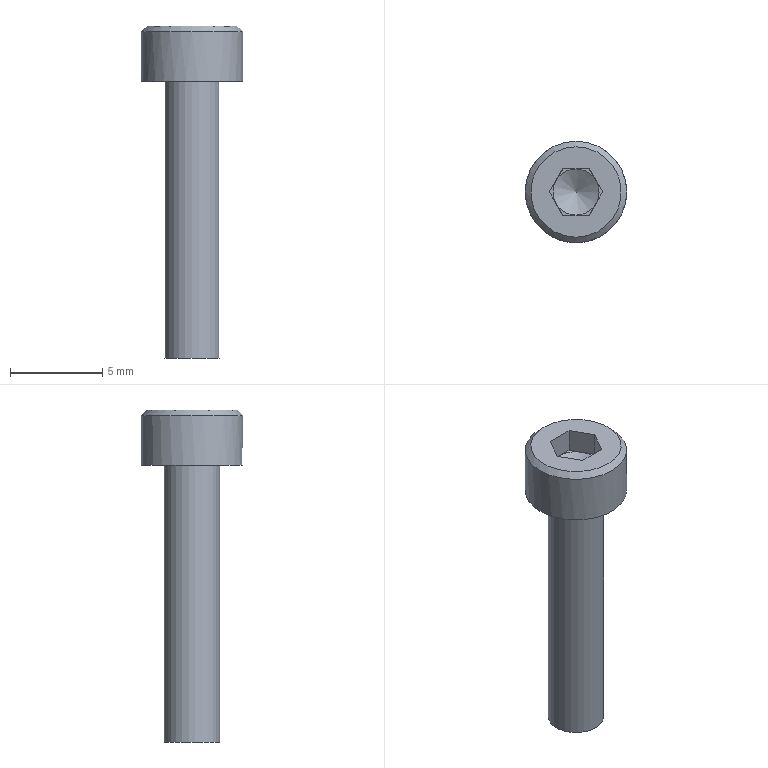Part | NX | features 5003_342_CB3-15 2 | 1 solid | 19 faces | box 5.5 x 5.5 x 18 mm | volume 168.289 mm3 | plane 15 | cylinder 2 | cone 2 | commonest cylinder face diameters 3 x1 5.5 x1
STEP:
#1=CARTESIAN_POINT('',(133.525,-558.45,-190.8));
#2=VERTEX_POINT('',#1);
#3=CARTESIAN_POINT('',(133.525,-556.,-190.8));
#4=DIRECTION('',(0.,0.,-1.));
#5=DIRECTION('',(0.,-1.,0.));
#6=AXIS2_PLACEMENT_3D('',#3,#4,#5);
#7=CIRCLE('',#6,2.45);
#8=EDGE_CURVE('',#2,#2,#7,.F.);
#9=ORIENTED_EDGE('',*,*,#8,.T.);
#10=EDGE_LOOP('',(#9));
#11=FACE_BOUND('',#10,.T.);
#12=CARTESIAN_POINT('',(134.968,-556.,-190.8));
#13=VERTEX_POINT('',#12);
#14=CARTESIAN_POINT('',(134.247,-554.75,-190.8));
#15=VERTEX_POINT('',#14);
#16=CARTESIAN_POINT('',(134.968,-556.,-190.8));
#17=DIRECTION('',(-0.5,0.866,0.));
#18=VECTOR('',#17,1000.);
#19=LINE('',#16,#18);
#20=EDGE_CURVE('',#13,#15,#19,.T.);
#21=ORIENTED_EDGE('',*,*,#20,.F.);
#22=CARTESIAN_POINT('',(134.247,-557.25,-190.8));
#23=VERTEX_POINT('',#22);
#24=CARTESIAN_POINT('',(134.247,-557.25,-190.8));
#25=DIRECTION('',(0.5,0.866,0.));
#26=VECTOR('',#25,1000.);
#27=LINE('',#24,#26);
#28=EDGE_CURVE('',#23,#13,#27,.T.);
#29=ORIENTED_EDGE('',*,*,#28,.F.);
#30=CARTESIAN_POINT('',(132.803,-557.25,-190.8));
#31=VERTEX_POINT('',#30);
#32=CARTESIAN_POINT('',(132.803,-557.25,-190.8));
#33=DIRECTION('',(1.,0.,0.));
#34=VECTOR('',#33,1000.);
#35=LINE('',#32,#34);
#36=EDGE_CURVE('',#31,#23,#35,.T.);
#37=ORIENTED_EDGE('',*,*,#36,.F.);
#38=CARTESIAN_POINT('',(132.082,-556.,-190.8));
#39=VERTEX_POINT('',#38);
#40=CARTESIAN_POINT('',(132.082,-556.,-190.8));
#41=DIRECTION('',(0.5,-0.866,0.));
#42=VECTOR('',#41,1000.);
#43=LINE('',#40,#42);
#44=EDGE_CURVE('',#39,#31,#43,.T.);
#45=ORIENTED_EDGE('',*,*,#44,.F.);
#46=CARTESIAN_POINT('',(132.803,-554.75,-190.8));
#47=VERTEX_POINT('',#46);
#48=CARTESIAN_POINT('',(132.803,-554.75,-190.8));
#49=DIRECTION('',(-0.5,-0.866,0.));
#50=VECTOR('',#49,1000.);
#51=LINE('',#48,#50);
#52=EDGE_CURVE('',#47,#39,#51,.T.);
#53=ORIENTED_EDGE('',*,*,#52,.F.);
#54=CARTESIAN_POINT('',(134.247,-554.75,-190.8));
#55=DIRECTION('',(-1.,0.,0.));
#56=VECTOR('',#55,1000.);
#57=LINE('',#54,#56);
#58=EDGE_CURVE('',#15,#47,#57,.T.);
#59=ORIENTED_EDGE('',*,*,#58,.F.);
#60=EDGE_LOOP('',(#21,#29,#37,#45,#53,#59));
#61=FACE_BOUND('',#60,.T.);
#62=CARTESIAN_POINT('',(130.775,-556.,-190.8));
#63=DIRECTION('',(0.,0.,-1.));
#64=DIRECTION('',(0.,-1.,0.));
#65=AXIS2_PLACEMENT_3D('',#62,#63,#64);
#66=PLANE('',#65);
#67=ADVANCED_FACE('',(#11,#61),#66,.F.);
#68=CARTESIAN_POINT('',(133.525,-554.5,-208.8));
#69=VERTEX_POINT('',#68);
#70=CARTESIAN_POINT('',(133.525,-556.,-208.8));
#71=DIRECTION('',(0.,0.,1.));
#72=DIRECTION('',(0.,1.,0.));
#73=AXIS2_PLACEMENT_3D('',#70,#71,#72);
#74=CIRCLE('',#73,1.5);
#75=EDGE_CURVE('',#69,#69,#74,.T.);
#76=ORIENTED_EDGE('',*,*,#75,.F.);
#77=EDGE_LOOP('',(#76));
#78=FACE_BOUND('',#77,.T.);
#79=CARTESIAN_POINT('',(133.525,-556.,-208.8));
#80=DIRECTION('',(0.,0.,1.));
#81=DIRECTION('',(0.,1.,0.));
#82=AXIS2_PLACEMENT_3D('',#79,#80,#81);
#83=PLANE('',#82);
#84=ADVANCED_FACE('',(#78),#83,.F.);
#85=CARTESIAN_POINT('',(133.525,-554.5,-193.8));
#86=VERTEX_POINT('',#85);
#87=CARTESIAN_POINT('',(133.525,-556.,-193.8));
#88=DIRECTION('',(0.,0.,1.));
#89=DIRECTION('',(0.,1.,0.));
#90=AXIS2_PLACEMENT_3D('',#87,#88,#89);
#91=CIRCLE('',#90,1.5);
#92=EDGE_CURVE('',#86,#86,#91,.T.);
#93=ORIENTED_EDGE('',*,*,#92,.F.);
#94=EDGE_LOOP('',(#93));
#95=FACE_BOUND('',#94,.T.);
#96=ORIENTED_EDGE('',*,*,#75,.T.);
#97=EDGE_LOOP('',(#96));
#98=FACE_BOUND('',#97,.T.);
#99=CARTESIAN_POINT('',(133.525,-556.,-190.8));
#100=DIRECTION('',(0.,0.,1.));
#101=DIRECTION('',(0.,1.,0.));
#102=AXIS2_PLACEMENT_3D('',#99,#100,#101);
#103=CYLINDRICAL_SURFACE('',#102,1.5);
#104=ADVANCED_FACE('',(#95,#98),#103,.T.);
#105=CARTESIAN_POINT('',(133.525,-553.25,-193.8));
#106=VERTEX_POINT('',#105);
#107=CARTESIAN_POINT('',(133.525,-556.,-193.8));
#108=DIRECTION('',(0.,0.,1.));
#109=DIRECTION('',(0.,1.,0.));
#110=AXIS2_PLACEMENT_3D('',#107,#108,#109);
#111=CIRCLE('',#110,2.75);
#112=EDGE_CURVE('',#106,#106,#111,.T.);
#113=ORIENTED_EDGE('',*,*,#112,.F.);
#114=EDGE_LOOP('',(#113));
#115=FACE_BOUND('',#114,.T.);
#116=ORIENTED_EDGE('',*,*,#92,.T.);
#117=EDGE_LOOP('',(#116));
#118=FACE_BOUND('',#117,.T.);
#119=CARTESIAN_POINT('',(132.025,-556.,-193.8));
#120=DIRECTION('',(0.,0.,1.));
#121=DIRECTION('',(0.,1.,0.));
#122=AXIS2_PLACEMENT_3D('',#119,#120,#121);
#123=PLANE('',#122);
#124=ADVANCED_FACE('',(#115,#118),#123,.F.);
#125=CARTESIAN_POINT('',(133.525,-558.75,-191.1));
#126=VERTEX_POINT('',#125);
#127=CARTESIAN_POINT('',(133.525,-556.,-191.1));
#128=DIRECTION('',(0.,0.,-1.));
#129=DIRECTION('',(0.,-1.,0.));
#130=AXIS2_PLACEMENT_3D('',#127,#128,#129);
#131=CIRCLE('',#130,2.75);
#132=EDGE_CURVE('',#126,#126,#131,.T.);
#133=ORIENTED_EDGE('',*,*,#132,.T.);
#134=EDGE_LOOP('',(#133));
#135=FACE_BOUND('',#134,.T.);
#136=ORIENTED_EDGE('',*,*,#112,.T.);
#137=EDGE_LOOP('',(#136));
#138=FACE_BOUND('',#137,.T.);
#139=CARTESIAN_POINT('',(133.525,-556.,-190.8));
#140=DIRECTION('',(0.,0.,1.));
#141=DIRECTION('',(0.,1.,0.));
#142=AXIS2_PLACEMENT_3D('',#139,#140,#141);
#143=CYLINDRICAL_SURFACE('',#142,2.75);
#144=ADVANCED_FACE('',(#135,#138),#143,.T.);
#145=ORIENTED_EDGE('',*,*,#132,.F.);
#146=EDGE_LOOP('',(#145));
#147=FACE_BOUND('',#146,.T.);
#148=ORIENTED_EDGE('',*,*,#8,.F.);
#149=EDGE_LOOP('',(#148));
#150=FACE_BOUND('',#149,.T.);
#151=CARTESIAN_POINT('',(133.525,-556.,-190.8));
#152=DIRECTION('',(0.,0.,-1.));
#153=DIRECTION('',(0.,-1.,0.));
#154=AXIS2_PLACEMENT_3D('',#151,#152,#153);
#155=CONICAL_SURFACE('',#154,2.45,0.7854);
#156=ADVANCED_FACE('',(#147,#150),#155,.T.);
#157=CARTESIAN_POINT('',(134.247,-557.25,-192.1));
#158=VERTEX_POINT('',#157);
#159=CARTESIAN_POINT('',(134.608,-556.625,-192.1));
#160=VERTEX_POINT('',#159);
#161=CARTESIAN_POINT('',(134.247,-557.25,-192.1));
#162=DIRECTION('',(0.5,0.866,0.));
#163=VECTOR('',#162,1000.);
#164=LINE('',#161,#163);
#165=EDGE_CURVE('',#158,#160,#164,.T.);
#166=ORIENTED_EDGE('',*,*,#165,.F.);
#167=CARTESIAN_POINT('',(134.247,-557.25,-192.1));
#168=DIRECTION('',(0.,0.,1.));
#169=VECTOR('',#168,1000.);
#170=LINE('',#167,#169);
#171=EDGE_CURVE('',#158,#23,#170,.T.);
#172=ORIENTED_EDGE('',*,*,#171,.T.);
#173=ORIENTED_EDGE('',*,*,#28,.T.);
#174=CARTESIAN_POINT('',(134.968,-556.,-192.1));
#175=VERTEX_POINT('',#174);
#176=CARTESIAN_POINT('',(134.968,-556.,-192.1));
#177=DIRECTION('',(0.,0.,1.));
#178=VECTOR('',#177,1000.);
#179=LINE('',#176,#178);
#180=EDGE_CURVE('',#175,#13,#179,.T.);
#181=ORIENTED_EDGE('',*,*,#180,.F.);
#182=CARTESIAN_POINT('',(134.247,-557.25,-192.1));
#183=DIRECTION('',(0.5,0.866,0.));
#184=VECTOR('',#183,1000.);
#185=LINE('',#182,#184);
#186=EDGE_CURVE('',#160,#175,#185,.T.);
#187=ORIENTED_EDGE('',*,*,#186,.F.);
#188=EDGE_LOOP('',(#166,#172,#173,#181,#187));
#189=FACE_BOUND('',#188,.T.);
#190=CARTESIAN_POINT('',(134.247,-557.25,-192.1));
#191=DIRECTION('',(0.866,-0.5,0.));
#192=DIRECTION('',(-0.5,-0.866,0.));
#193=AXIS2_PLACEMENT_3D('',#190,#191,#192);
#194=PLANE('',#193);
#195=ADVANCED_FACE('',(#189),#194,.F.);
#196=CARTESIAN_POINT('',(132.803,-557.25,-192.1));
#197=VERTEX_POINT('',#196);
#198=CARTESIAN_POINT('',(133.525,-557.25,-192.1));
#199=VERTEX_POINT('',#198);
#200=CARTESIAN_POINT('',(132.803,-557.25,-192.1));
#201=DIRECTION('',(1.,0.,0.));
#202=VECTOR('',#201,1000.);
#203=LINE('',#200,#202);
#204=EDGE_CURVE('',#197,#199,#203,.T.);
#205=ORIENTED_EDGE('',*,*,#204,.F.);
#206=CARTESIAN_POINT('',(132.803,-557.25,-192.1));
#207=DIRECTION('',(0.,0.,1.));
#208=VECTOR('',#207,1000.);
#209=LINE('',#206,#208);
#210=EDGE_CURVE('',#197,#31,#209,.T.);
#211=ORIENTED_EDGE('',*,*,#210,.T.);
#212=ORIENTED_EDGE('',*,*,#36,.T.);
#213=ORIENTED_EDGE('',*,*,#171,.F.);
#214=CARTESIAN_POINT('',(132.803,-557.25,-192.1));
#215=DIRECTION('',(1.,0.,0.));
#216=VECTOR('',#215,1000.);
#217=LINE('',#214,#216);
#218=EDGE_CURVE('',#199,#158,#217,.T.);
#219=ORIENTED_EDGE('',*,*,#218,.F.);
#220=EDGE_LOOP('',(#205,#211,#212,#213,#219));
#221=FACE_BOUND('',#220,.T.);
#222=CARTESIAN_POINT('',(132.803,-557.25,-192.1));
#223=DIRECTION('',(0.,-1.,0.));
#224=DIRECTION('',(-1.,0.,0.));
#225=AXIS2_PLACEMENT_3D('',#222,#223,#224);
#226=PLANE('',#225);
#227=ADVANCED_FACE('',(#221),#226,.F.);
#228=CARTESIAN_POINT('',(132.082,-556.,-192.1));
#229=VERTEX_POINT('',#228);
#230=CARTESIAN_POINT('',(132.442,-556.625,-192.1));
#231=VERTEX_POINT('',#230);
#232=CARTESIAN_POINT('',(132.082,-556.,-192.1));
#233=DIRECTION('',(0.5,-0.866,0.));
#234=VECTOR('',#233,1000.);
#235=LINE('',#232,#234);
#236=EDGE_CURVE('',#229,#231,#235,.T.);
#237=ORIENTED_EDGE('',*,*,#236,.F.);
#238=CARTESIAN_POINT('',(132.082,-556.,-192.1));
#239=DIRECTION('',(0.,0.,1.));
#240=VECTOR('',#239,1000.);
#241=LINE('',#238,#240);
#242=EDGE_CURVE('',#229,#39,#241,.T.);
#243=ORIENTED_EDGE('',*,*,#242,.T.);
#244=ORIENTED_EDGE('',*,*,#44,.T.);
#245=ORIENTED_EDGE('',*,*,#210,.F.);
#246=CARTESIAN_POINT('',(132.082,-556.,-192.1));
#247=DIRECTION('',(0.5,-0.866,0.));
#248=VECTOR('',#247,1000.);
#249=LINE('',#246,#248);
#250=EDGE_CURVE('',#231,#197,#249,.T.);
#251=ORIENTED_EDGE('',*,*,#250,.F.);
#252=EDGE_LOOP('',(#237,#243,#244,#245,#251));
#253=FACE_BOUND('',#252,.T.);
#254=CARTESIAN_POINT('',(132.082,-556.,-192.1));
#255=DIRECTION('',(-0.866,-0.5,0.));
#256=DIRECTION('',(-0.5,0.866,0.));
#257=AXIS2_PLACEMENT_3D('',#254,#255,#256);
#258=PLANE('',#257);
#259=ADVANCED_FACE('',(#253),#258,.F.);
#260=CARTESIAN_POINT('',(132.803,-554.75,-192.1));
#261=VERTEX_POINT('',#260);
#262=CARTESIAN_POINT('',(132.442,-555.375,-192.1));
#263=VERTEX_POINT('',#262);
#264=CARTESIAN_POINT('',(132.803,-554.75,-192.1));
#265=DIRECTION('',(-0.5,-0.866,0.));
#266=VECTOR('',#265,1000.);
#267=LINE('',#264,#266);
#268=EDGE_CURVE('',#261,#263,#267,.T.);
#269=ORIENTED_EDGE('',*,*,#268,.F.);
#270=CARTESIAN_POINT('',(132.803,-554.75,-192.1));
#271=DIRECTION('',(0.,0.,1.));
#272=VECTOR('',#271,1000.);
#273=LINE('',#270,#272);
#274=EDGE_CURVE('',#261,#47,#273,.T.);
#275=ORIENTED_EDGE('',*,*,#274,.T.);
#276=ORIENTED_EDGE('',*,*,#52,.T.);
#277=ORIENTED_EDGE('',*,*,#242,.F.);
#278=CARTESIAN_POINT('',(132.803,-554.75,-192.1));
#279=DIRECTION('',(-0.5,-0.866,0.));
#280=VECTOR('',#279,1000.);
#281=LINE('',#278,#280);
#282=EDGE_CURVE('',#263,#229,#281,.T.);
#283=ORIENTED_EDGE('',*,*,#282,.F.);
#284=EDGE_LOOP('',(#269,#275,#276,#277,#283));
#285=FACE_BOUND('',#284,.T.);
#286=CARTESIAN_POINT('',(132.803,-554.75,-192.1));
#287=DIRECTION('',(-0.866,0.5,0.));
#288=DIRECTION('',(0.5,0.866,0.));
#289=AXIS2_PLACEMENT_3D('',#286,#287,#288);
#290=PLANE('',#289);
#291=ADVANCED_FACE('',(#285),#290,.F.);
#292=CARTESIAN_POINT('',(134.247,-554.75,-192.1));
#293=VERTEX_POINT('',#292);
#294=CARTESIAN_POINT('',(133.525,-554.75,-192.1));
#295=VERTEX_POINT('',#294);
#296=CARTESIAN_POINT('',(134.247,-554.75,-192.1));
#297=DIRECTION('',(-1.,0.,0.));
#298=VECTOR('',#297,1000.);
#299=LINE('',#296,#298);
#300=EDGE_CURVE('',#293,#295,#299,.T.);
#301=ORIENTED_EDGE('',*,*,#300,.F.);
#302=CARTESIAN_POINT('',(134.247,-554.75,-192.1));
#303=DIRECTION('',(0.,0.,1.));
#304=VECTOR('',#303,1000.);
#305=LINE('',#302,#304);
#306=EDGE_CURVE('',#293,#15,#305,.T.);
#307=ORIENTED_EDGE('',*,*,#306,.T.);
#308=ORIENTED_EDGE('',*,*,#58,.T.);
#309=ORIENTED_EDGE('',*,*,#274,.F.);
#310=CARTESIAN_POINT('',(134.247,-554.75,-192.1));
#311=DIRECTION('',(-1.,0.,0.));
#312=VECTOR('',#311,1000.);
#313=LINE('',#310,#312);
#314=EDGE_CURVE('',#295,#261,#313,.T.);
#315=ORIENTED_EDGE('',*,*,#314,.F.);
#316=EDGE_LOOP('',(#301,#307,#308,#309,#315));
#317=FACE_BOUND('',#316,.T.);
#318=CARTESIAN_POINT('',(134.247,-554.75,-192.1));
#319=DIRECTION('',(0.,1.,0.));
#320=DIRECTION('',(0.,0.,-1.));
#321=AXIS2_PLACEMENT_3D('',#318,#319,#320);
#322=PLANE('',#321);
#323=ADVANCED_FACE('',(#317),#322,.F.);
#324=CARTESIAN_POINT('',(134.608,-555.375,-192.1));
#325=VERTEX_POINT('',#324);
#326=CARTESIAN_POINT('',(134.968,-556.,-192.1));
#327=DIRECTION('',(-0.5,0.866,0.));
#328=VECTOR('',#327,1000.);
#329=LINE('',#326,#328);
#330=EDGE_CURVE('',#175,#325,#329,.T.);
#331=ORIENTED_EDGE('',*,*,#330,.F.);
#332=ORIENTED_EDGE('',*,*,#180,.T.);
#333=ORIENTED_EDGE('',*,*,#20,.T.);
#334=ORIENTED_EDGE('',*,*,#306,.F.);
#335=CARTESIAN_POINT('',(134.968,-556.,-192.1));
#336=DIRECTION('',(-0.5,0.866,0.));
#337=VECTOR('',#336,1000.);
#338=LINE('',#335,#337);
#339=EDGE_CURVE('',#325,#293,#338,.T.);
#340=ORIENTED_EDGE('',*,*,#339,.F.);
#341=EDGE_LOOP('',(#331,#332,#333,#334,#340));
#342=FACE_BOUND('',#341,.T.);
#343=CARTESIAN_POINT('',(134.968,-556.,-192.1));
#344=DIRECTION('',(0.866,0.5,0.));
#345=DIRECTION('',(0.5,-0.866,0.));
#346=AXIS2_PLACEMENT_3D('',#343,#344,#345);
#347=PLANE('',#346);
#348=ADVANCED_FACE('',(#342),#347,.F.);
#349=ORIENTED_EDGE('',*,*,#314,.T.);
#350=ORIENTED_EDGE('',*,*,#268,.T.);
#351=CARTESIAN_POINT('',(133.525,-556.,-192.1));
#352=DIRECTION('',(0.,0.,1.));
#353=DIRECTION('',(1.,0.,0.));
#354=AXIS2_PLACEMENT_3D('',#351,#352,#353);
#355=CIRCLE('',#354,1.25);
#356=EDGE_CURVE('',#295,#263,#355,.T.);
#357=ORIENTED_EDGE('',*,*,#356,.F.);
#358=EDGE_LOOP('',(#349,#350,#357));
#359=FACE_BOUND('',#358,.T.);
#360=CARTESIAN_POINT('',(133.525,-556.,-192.1));
#361=DIRECTION('',(0.,0.,1.));
#362=DIRECTION('',(0.,1.,0.));
#363=AXIS2_PLACEMENT_3D('',#360,#361,#362);
#364=PLANE('',#363);
#365=ADVANCED_FACE('',(#359),#364,.T.);
#366=ORIENTED_EDGE('',*,*,#282,.T.);
#367=ORIENTED_EDGE('',*,*,#236,.T.);
#368=CARTESIAN_POINT('',(133.525,-556.,-192.1));
#369=DIRECTION('',(0.,0.,1.));
#370=DIRECTION('',(1.,0.,0.));
#371=AXIS2_PLACEMENT_3D('',#368,#369,#370);
#372=CIRCLE('',#371,1.25);
#373=EDGE_CURVE('',#263,#231,#372,.T.);
#374=ORIENTED_EDGE('',*,*,#373,.F.);
#375=EDGE_LOOP('',(#366,#367,#374));
#376=FACE_BOUND('',#375,.T.);
#377=CARTESIAN_POINT('',(133.525,-556.,-192.1));
#378=DIRECTION('',(0.,0.,1.));
#379=DIRECTION('',(0.,1.,0.));
#380=AXIS2_PLACEMENT_3D('',#377,#378,#379);
#381=PLANE('',#380);
#382=ADVANCED_FACE('',(#376),#381,.T.);
#383=ORIENTED_EDGE('',*,*,#250,.T.);
#384=ORIENTED_EDGE('',*,*,#204,.T.);
#385=CARTESIAN_POINT('',(133.525,-556.,-192.1));
#386=DIRECTION('',(0.,0.,1.));
#387=DIRECTION('',(1.,0.,0.));
#388=AXIS2_PLACEMENT_3D('',#385,#386,#387);
#389=CIRCLE('',#388,1.25);
#390=EDGE_CURVE('',#231,#199,#389,.T.);
#391=ORIENTED_EDGE('',*,*,#390,.F.);
#392=EDGE_LOOP('',(#383,#384,#391));
#393=FACE_BOUND('',#392,.T.);
#394=CARTESIAN_POINT('',(133.525,-556.,-192.1));
#395=DIRECTION('',(0.,0.,1.));
#396=DIRECTION('',(0.,1.,0.));
#397=AXIS2_PLACEMENT_3D('',#394,#395,#396);
#398=PLANE('',#397);
#399=ADVANCED_FACE('',(#393),#398,.T.);
#400=ORIENTED_EDGE('',*,*,#218,.T.);
#401=ORIENTED_EDGE('',*,*,#165,.T.);
#402=CARTESIAN_POINT('',(133.525,-556.,-192.1));
#403=DIRECTION('',(0.,0.,1.));
#404=DIRECTION('',(1.,0.,0.));
#405=AXIS2_PLACEMENT_3D('',#402,#403,#404);
#406=CIRCLE('',#405,1.25);
#407=EDGE_CURVE('',#199,#160,#406,.T.);
#408=ORIENTED_EDGE('',*,*,#407,.F.);
#409=EDGE_LOOP('',(#400,#401,#408));
#410=FACE_BOUND('',#409,.T.);
#411=CARTESIAN_POINT('',(133.525,-556.,-192.1));
#412=DIRECTION('',(0.,0.,1.));
#413=DIRECTION('',(0.,1.,0.));
#414=AXIS2_PLACEMENT_3D('',#411,#412,#413);
#415=PLANE('',#414);
#416=ADVANCED_FACE('',(#410),#415,.T.);
#417=ORIENTED_EDGE('',*,*,#186,.T.);
#418=ORIENTED_EDGE('',*,*,#330,.T.);
#419=CARTESIAN_POINT('',(133.525,-556.,-192.1));
#420=DIRECTION('',(0.,0.,1.));
#421=DIRECTION('',(1.,0.,0.));
#422=AXIS2_PLACEMENT_3D('',#419,#420,#421);
#423=CIRCLE('',#422,1.25);
#424=EDGE_CURVE('',#160,#325,#423,.T.);
#425=ORIENTED_EDGE('',*,*,#424,.F.);
#426=EDGE_LOOP('',(#417,#418,#425));
#427=FACE_BOUND('',#426,.T.);
#428=CARTESIAN_POINT('',(133.525,-556.,-192.1));
#429=DIRECTION('',(0.,0.,1.));
#430=DIRECTION('',(0.,1.,0.));
#431=AXIS2_PLACEMENT_3D('',#428,#429,#430);
#432=PLANE('',#431);
#433=ADVANCED_FACE('',(#427),#432,.T.);
#434=ORIENTED_EDGE('',*,*,#339,.T.);
#435=ORIENTED_EDGE('',*,*,#300,.T.);
#436=CARTESIAN_POINT('',(133.525,-556.,-192.1));
#437=DIRECTION('',(0.,0.,1.));
#438=DIRECTION('',(1.,0.,0.));
#439=AXIS2_PLACEMENT_3D('',#436,#437,#438);
#440=CIRCLE('',#439,1.25);
#441=EDGE_CURVE('',#325,#295,#440,.T.);
#442=ORIENTED_EDGE('',*,*,#441,.F.);
#443=EDGE_LOOP('',(#434,#435,#442));
#444=FACE_BOUND('',#443,.T.);
#445=CARTESIAN_POINT('',(133.525,-556.,-192.1));
#446=DIRECTION('',(0.,0.,1.));
#447=DIRECTION('',(0.,1.,0.));
#448=AXIS2_PLACEMENT_3D('',#445,#446,#447);
#449=PLANE('',#448);
#450=ADVANCED_FACE('',(#444),#449,.T.);
#451=ORIENTED_EDGE('',*,*,#441,.T.);
#452=ORIENTED_EDGE('',*,*,#356,.T.);
#453=ORIENTED_EDGE('',*,*,#373,.T.);
#454=ORIENTED_EDGE('',*,*,#390,.T.);
#455=ORIENTED_EDGE('',*,*,#407,.T.);
#456=ORIENTED_EDGE('',*,*,#424,.T.);
#457=EDGE_LOOP('',(#451,#452,#453,#454,#455,#456));
#458=FACE_BOUND('',#457,.T.);
#459=CARTESIAN_POINT('',(133.525,-556.,-192.851));
#460=VERTEX_POINT('',#459);
#461=VERTEX_LOOP('',#460);
#462=FACE_BOUND('',#461,.T.);
#463=CARTESIAN_POINT('',(133.525,-556.,-192.851));
#464=DIRECTION('',(0.,0.,1.));
#465=DIRECTION('',(1.,0.,0.));
#466=AXIS2_PLACEMENT_3D('',#463,#464,#465);
#467=CONICAL_SURFACE('',#466,0.,1.03);
#468=ADVANCED_FACE('',(#458,#462),#467,.F.);
#469=CLOSED_SHELL('',(#67,#84,#104,#124,#144,#156,#195,#227,#259,#291,#323,#348,#365,#382,#399,#416,#433,#450,#468));
#470=MANIFOLD_SOLID_BREP('',#469);
#471=(LENGTH_UNIT()NAMED_UNIT(*)SI_UNIT(.MILLI.,.METRE.));
#472=UNCERTAINTY_MEASURE_WITH_UNIT(LENGTH_MEASURE(0.00001),#471,'','');
#473=(NAMED_UNIT(*)PLANE_ANGLE_UNIT()SI_UNIT($,.RADIAN.));
#474=(NAMED_UNIT(*)SI_UNIT($,.STERADIAN.)SOLID_ANGLE_UNIT());
#475=(GEOMETRIC_REPRESENTATION_CONTEXT(3)GLOBAL_UNCERTAINTY_ASSIGNED_CONTEXT((#472))GLOBAL_UNIT_ASSIGNED_CONTEXT((#471,#473,#474))REPRESENTATION_CONTEXT('',''));
#476=ADVANCED_BREP_SHAPE_REPRESENTATION('',(#470),#475);